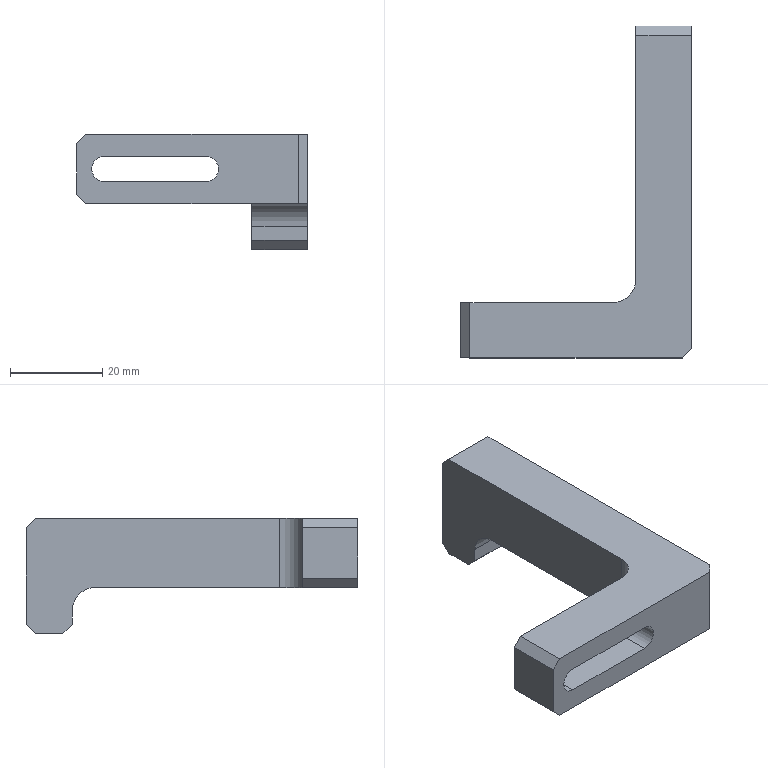NC program | NX | posted with a generic post | part box 50 x 72 x 25 mm
Whole program:
N10 G17 G21 G94 G90
(PLANAR_MILL , TOOL : D10)
N12 T15 M6
N14 G54
N16 G17 G0 G90 X-47. Y-7.8 B0. C0. S9500 M3
N18 G43 Z30. H15
N20 Z8.
N22 G94 G1 Z5. F2000.
N24 X-36.
N26 X18.8
N28 Y25.
N30 Y36.
N32 Z8.
N34 G0 Z16.
N36 X-47. Y-7.8
N38 Z7.
N40 G1 Z4.
N42 X-36.
N44 X18.8
N46 Y25.
N48 Y36.
N50 Z7.
N52 G0 Z15.
N54 X-47. Y-7.8
N56 Z6.
N58 G1 Z3.
N60 X-36.
N62 X18.8
N64 Y25.
N66 Y36.
N68 Z6.
N70 G0 Z14.
N72 X-47. Y-7.8
N74 Z5.
N76 G1 Z2.
N78 X-36.
N80 X18.8
N82 Y25.
N84 Y36.
N86 Z5.
N88 G0 Z13.
N90 X-47. Y-7.8
N92 Z4.
N94 G1 Z1.
N96 X-36.
N98 X18.8
N100 Y25.
N102 Y36.
N104 Z4.
N106 G0 Z12.
N108 X-47. Y-7.8
N110 Z3.
N112 G1 Z0.
N114 X-36.
N116 X18.8
N118 Y25.
N120 Y36.
N122 Z3.
N124 G0 Z11.
N126 X-47. Y-7.8
N128 Z2.5
N130 G1 Z-0.5
N132 X-36.
N134 X18.8
N136 Y25.
N138 Y36.
N140 Z2.5
N142 G0 Z30.
N144 M5
(FLOOR_WALL_COPY , TOOL : D80)
N146 T19 M6
N148 G54
N150 G17 G0 G90 X81. Y0. B0. C0. S6500 M3
N152 G43 Z30. H19
N154 Z7.
N156 G94 G1 Z4. F1500.
N158 X78.
N160 X-78.
N162 X-81.
N164 Z7.
N166 G0 Z30.
N168 X81.
N170 Z6.
N172 G1 Z3.
N174 X78.
N176 X-78.
N178 X-81.
N180 Z6.
N182 G0 Z30.
N184 X81.
N186 Z5.
N188 G1 Z2.
N190 X78.
N192 X-78.
N194 X-81.
N196 Z5.
N198 G0 Z30.
N200 X81.
N202 Z4.
N204 G1 Z1.
N206 X78.
N208 X-78.
N210 X-81.
N212 Z4.
N214 G0 Z30.
N216 X81.
N218 Z3.
N220 G1 Z0.
N222 X78.
N224 X-78.
N226 X-81.
N228 Z3.
N230 G0 Z30.
N232 M5
(PLANAR_MILL_COPY_COPY_COPY_COPY_1 , TOOL : D6A45)
N234 T01 M6
N236 G54
N238 G17 G0 G90 X-16.908 Y-10.687 B0. C0. S9500 M3
N240 G43 Z30. H1
N242 Z-9.5
N244 G94 G1 Z-11. F1250.
N246 X-17.357 Y-11.135
N248 G3 X-17.618 Y-12.1 R1.
N250 G1 X19.
N252 G3 X23.1 Y-8. R4.1
N254 G1 Y22.9
N256 G2 X24.1 Y23.9 R1.
N258 G1 X35.9
N260 G2 X36.9 Y22.9 R1.
N262 G1 Y-22.959
N264 G2 X36.607 Y-23.666 R1.
N266 G1 X34.666 Y-25.607
N268 G2 X33.959 Y-25.9 R1.
N270 G1 X-17.618
N272 G3 X-17.357 Y-26.865 R1.
N274 G1 X-16.908 Y-27.313
N276 Z-9.5
N278 G0 Z30.
N280 M5
N282 M2